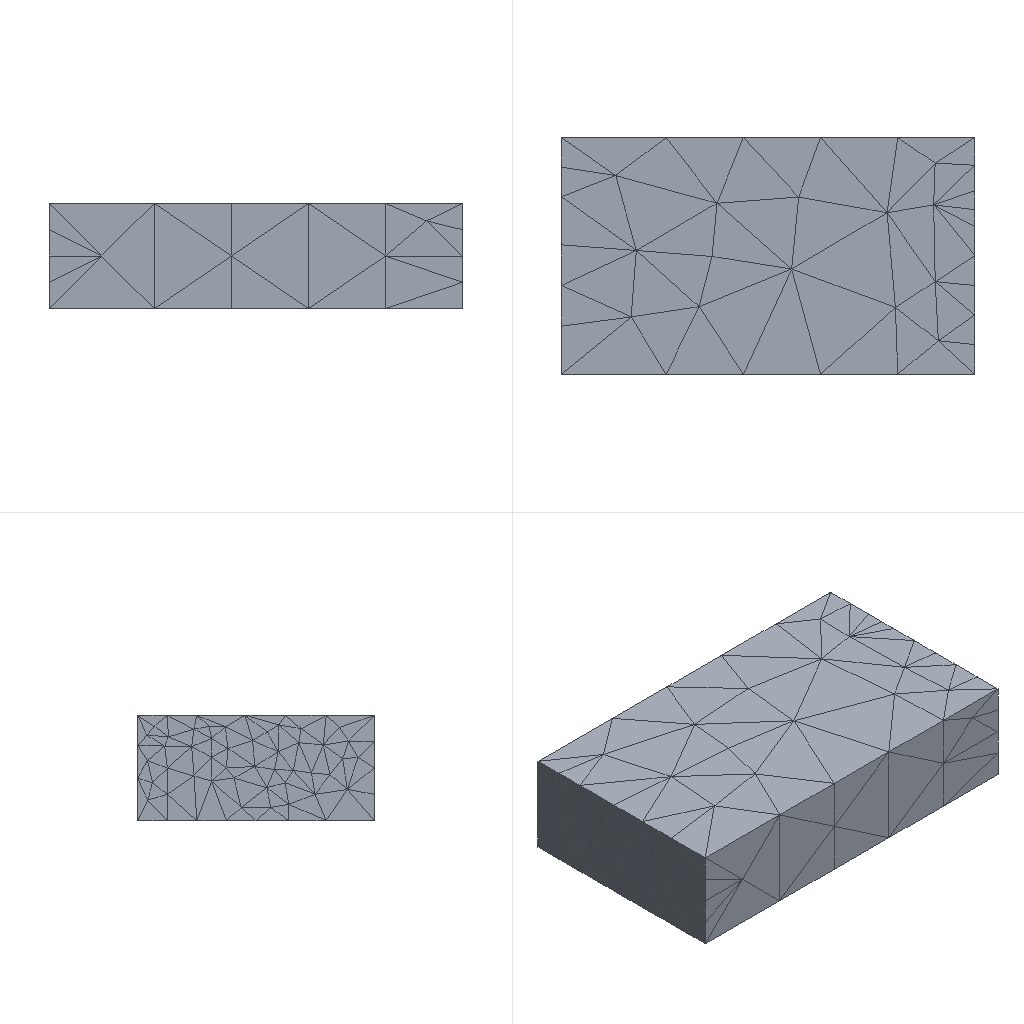Simulation study | ansys electronics desktop
Set-up summary:
category,name,step,type,value,unit,region
solver,ansys_electronics_desktop
units,length mm,,stated,model units
analysis,M03,,HFSS Modal Network,design_type=HFSS
setup,Setup1,M03,HfssDriven,frequency=10GHz; max_passes=2; max_delta_s=0.08
sweep,Sweep1,Setup1,Interpolating,8GHz..12GHz n=11 step=
mesh,nodes,,,n/a (no mesh stored)
mesh,elements,,,n/a (no mesh stored)
material,vacuum,,permittivity,1
load,P1,M03,wave port,,,objects 34
load,P2,M03,wave port,,,objects 46
bc,PerfE_6CU0FH,M03,perfect e,,,objects 58
bc,PerfE_674NPD,M03,perfect e,,,objects 70
bc,PerfE_5CT5JI,M03,perfect e,,,objects 82
bc,PerfE_WCUXQC,M03,perfect e,,,objects 94
Ansys Electronics Desktop project file, long lists of numbers shortened, first 681 of 3480 lines:
$begin 'AnsoftProject'
	Created='Wed Sep 30 18:28:02 2026'
	Product='ElectronicsDesktop'
	FileOwnedByWorkbench=false
	$begin 'Desktop'
		Version(2026, 1)
		InfrastructureVersion(1, 0)
		$begin 'FactoryHeader'
			$begin 'geometry3deditor'
				KernelVersion(2, 0)
				ProjectContainsGeometry3D='1'
			$end 'geometry3deditor'
		$end 'FactoryHeader'
	$end 'Desktop'
	UsesAdvancedFeatures=false
	PreviewImageDesignId=1
	NextUniqueID=0
	MoveBackwards=false
	$begin 'HFSSEnvironment'
		Version(1, 0)
	$end 'HFSSEnvironment'
	$begin 'PlanarEMEnvironment'
		Version(1, 0)
	$end 'PlanarEMEnvironment'
	$begin 'Q3DEnvironment'
		Version(1, 0)
	$end 'Q3DEnvironment'
	$begin '2DExtractorEnvironment'
		Version(1, 0)
	$end '2DExtractorEnvironment'
	$begin 'NexximEnvironment'
		Version(1, 0)
	$end 'NexximEnvironment'
	$begin 'NexximNetlistEnvironment'
		Version(1, 0)
	$end 'NexximNetlistEnvironment'
	$begin 'EmitEnvironment'
		Version(1, 0)
	$end 'EmitEnvironment'
	$begin 'Maxwell3DEnvironment'
		Version(1, 0)
	$end 'Maxwell3DEnvironment'
	$begin 'Maxwell2DEnvironment'
		Version(1, 0)
	$end 'Maxwell2DEnvironment'
	$begin 'RMxprtEnvironment'
		Version(1, 0)
	$end 'RMxprtEnvironment'
	$begin 'MaxCirEnvironment'
		Version(1, 0)
	$end 'MaxCirEnvironment'
	$begin 'SimplorerEnvironment'
		Version(1, 0)
	$end 'SimplorerEnvironment'
	$begin 'IcepakEnvironment'
		Version(1, 0)
	$end 'IcepakEnvironment'
	$begin 'IcepakFEAEnvironment'
		Version(1, 0)
	$end 'IcepakFEAEnvironment'
	$begin 'SchematicEnvironment'
		Version(1, 0)
	$end 'SchematicEnvironment'
	$begin 'geometry3deditor'
		Version(1, 0)
	$end 'geometry3deditor'
	ReadVersion=12
	$begin 'DesignMgrEnvironment'
		CompInstCounter=1
		GPortCounter=0
		NetCounter=0
		Alias('Ieee;Simplorer Elements\\Ieee', 'Std;Simplorer Elements\\Std', 'Basic_VHDLAMS;Simplorer Elements\\Basic Elements VHDLAMS\\Basic Elements VHDLAMS', 'Digital_Elements;Simplorer Elements\\Digital Elements\\Digital Elements', 'Transformations;Simplorer Elements\\Tools\\Transformations\\Transformations', 'HEV_VHDLAMS;Simplorer Elements\\HEV VHDLAMS\\HEV VHDLAMS', 'automotive_vda;Simplorer Elem
	$end 'DesignMgrEnvironment'
	$begin 'ProjectDatasets'
		NextUniqueID=0
		MoveBackwards=false
		DatasetType='ProjectDatasetType'
		$begin 'DatasetDefinitions'
		$end 'DatasetDefinitions'
	$end 'ProjectDatasets'
	VariableOrders[0:]
	$begin 'Definitions'
		$begin 'Materials'
			$begin 'vacuum'
				CoordinateSystemType='Cartesian'
				BulkOrSurfaceType=1
				$begin 'PhysicsTypes'
					set('Electromagnetic')
				$end 'PhysicsTypes'
				$begin 'AttachedData'
					$begin 'MatAppearanceData'
						property_data='appearance_data'
						Red=230
						Green=230
						Blue=230
						Transparency=0.95
					$end 'MatAppearanceData'
				$end 'AttachedData'
				permittivity='1'
				ModTime=1499970477
				Library='Materials'
				LibLocation='SysLibrary'
				ModSinceLib=false
			$end 'vacuum'
		$end 'Materials'
		$begin 'SurfaceMaterials'
		$end 'SurfaceMaterials'
		$begin 'Scripts'
		$end 'Scripts'
		$begin 'AnsysComponents'
			NextUniqueID=0
			MoveBackwards=false
			$begin 'AnsysComponentDefinitions'
			$end 'AnsysComponentDefinitions'
		$end 'AnsysComponents'
		$begin 'Symbols'
			$begin 'M03'
				ModTime=1790764083
				Library=''
				ModSinceLib=false
				LibLocation='Project'
				HighestLevel=1
				Normalize=true
				InitialLevels(0, 1)
				$begin 'Graphics'
					Rect(0, 0, 0, 0, 0.00254, 0.00254, 0.00508, 0.00508, 0, 0, 0)
					Rect(0, 1, 0, 0, 0.0004233, 0.00254, 0.0004233, 0.0004233, 0, 0, 0)
				$end 'Graphics'
			$end 'M03'
		$end 'Symbols'
		$begin 'DefInfo'
			M03(1002, 0, 0, 0, '', 1790764083, '', 'M03', '', '', '', '', '', 'Design.bmp', '', 'Project', '', '', 1790764083, '', 0, 0)
		$end 'DefInfo'
		$begin 'Compdefs'
			$begin 'M03'
				Library=''
				CircuitEnv=0
				Refbase='U'
				NumParts=1
				ModSinceLib=true
				$begin 'Properties'
					TextProp('Representation', 'SRD', '', 'M03')
					TextProp('Owner', 'SRD', '', 'HFSS')
				$end 'Properties'
				CompExtID=6
				$begin 'Parameters'
					ButtonProp('CosimDefinition', 'D', '', 'Edit', 'Edit', 40501, ButtonPropClientData())
					MenuProp('CoSimulator', 'D', '', 'DefaultNetlist', 0)
				$end 'Parameters'
				$begin 'CosimDefinitions'
					$begin 'CosimDefinition'
						CosimulatorType=4
						CosimDefName='DefaultNetlist'
						IsDefinition=true
						Connect=true
						Data()
						GRef()
					$end 'CosimDefinition'
					DefaultCosim='DefaultNetlist'
				$end 'CosimDefinitions'
			$end 'M03'
		$end 'Compdefs'
	$end 'Definitions'
	DesignIDServer=2
	MoveBackwards=false
	$begin 'HFSSModel'
		RepRewriteV2=true
		Name='M03'
		DesignID=0
		'Use Advanced DC Extrapolation'=false
		'Use Power S'=false
		'Export FRTM After Simulation'=false
		'Export Rays After Simulation'=false
		'Export After Simulation'=false
		'Allow Material Override'=false
		'Calculate Lossy Dielectrics'=false
		'Perform Minimal validation'=false
		$begin 'TemperatureSettings'
			IncludeTemperatureDependence=false
			EnableFeedback=false
			Temperatures(6, '22cel', 34, '22cel', 46, '22cel', 58, '22cel', 70, '22cel', 82, '22cel', 94, '22cel')
		$end 'TemperatureSettings'
		ObjsEnabledForDeformation()
		'Port Validation Settings'='Standard'
		'Save Adaptive support files'=false
		SolutionType='HFSS Modal Network'
		$begin 'DrivenOptions'
			AutoOpen=false
		$end 'DrivenOptions'
		HasTransientSetups=false
		MaterialDensity=1
		MassOfTissue=1
		VoxelSize=1
		TissueObjectList=-1
		AverageSarMethod=0
		UseAutoDCThickness=true
		HaveZwaveSupport=true
		SolveInsideThreshold=100000
		RequireBodyFaceInfo=false
		$begin 'OutputVariable'
			NextUniqueID=0
			MoveBackwards=false
		$end 'OutputVariable'
		$begin 'ModelSetup'
			$begin 'DesignDatasets'
				NextUniqueID=0
				MoveBackwards=false
				DatasetType='DesignDatasetType'
				$begin 'DatasetDefinitions'
				$end 'DatasetDefinitions'
			$end 'DesignDatasets'
			VariableOrders[0:]
			$begin 'Editor3D Doc Preferences'
				BackgroundColorVersion=1
				'Plane Background'=0
				'Need Lights'=true
				'Ambient Light'=8355711
				'Num Lights'=1
				Light0[4: 16777215, 0.75, -0.15, -0.63]
				Ver=2
			$end 'Editor3D Doc Preferences'
			SnapMode=31
			WorkingCS=1
			$begin 'GeometryCore'
				BlockVersionID=3
				DataVersion=2
				NativeKernel='PARASOLID'
				NativeKernelVersionID=26
				Units='mm'
				ModelExtents=10000
				InstanceID=-1
				$begin 'ValidationOptions'
					EntityCheckLevel='Strict'
					IgnoreUnclassifiedObjects=false
					SkipIntersectionChecks=false
				$end 'ValidationOptions'
				ContainsGeomLinkUDM=false
				$begin 'GeometryOperations'
					BlockVersionID=2
					$begin 'AnsoftRangedIDServerManager'
						$begin 'AnsoftRangedIDServer'
							IDServerObjectTypeID=0
							IDServerRangeMin=0
							IDServerRangeMax=2146483647
							NextUniqueID=105
							MoveBackwards=false
						$end 'AnsoftRangedIDServer'
						$begin 'AnsoftRangedIDServer'
							IDServerObjectTypeID=1
							IDServerRangeMin=2146483648
							IDServerRangeMax=2146485547
							NextUniqueID=2146483654
							MoveBackwards=false
						$end 'AnsoftRangedIDServer'
					$end 'AnsoftRangedIDServerManager'
					StartBackGroundFaceID=2146483648
					$begin 'CoordinateSystems'
					$end 'CoordinateSystems'
					$begin 'OperandCSs'
					$end 'OperandCSs'
					$begin 'SubModelDefinitions'
					$end 'SubModelDefinitions'
					$begin 'Groups'
					$end 'Groups'
					$begin 'UserDefinedModels'
					$end 'UserDefinedModels'
					$begin 'OperandUserDefinedModels'
					$end 'OperandUserDefinedModels'
					$begin 'ToplevelParts'
						$begin 'GeometryPart'
							$begin 'Attributes'
								Name='WG'
								Flags=''
								Color='(230 230 230)'
								Transparency=0.8
								PartCoordinateSystem=1
								UDMId=-1
								GroupId=-1
								MaterialValue='"vacuum"'
								SurfaceMaterialValue='""'
								SolveInside=true
								ShellElement=false
								ShellElementThickness='0mm'
								ReferenceTemperature='20cel'
								IsMaterialEditable=true
								IsSurfaceMaterialEditable=true
								UseMaterialAppearance=false
								IsLightweight=false
								IsAlwaysHidden=false
							$end 'Attributes'
							$begin 'PhysicsAttributes'
								SuppressedForPhysics='False'
								SuppressedForPhysicsEditable=true
							$end 'PhysicsAttributes'
							$begin 'Operations'
								$begin 'Operation'
									OperationType='Box'
									ID=5
									ReferenceCoordSystemID=1
									$begin 'BoxParameters'
										KernelVersion=23
										XPosition='0mm'
										YPosition='0mm'
										ZPosition='0mm'
										XSize='40mm'
										YSize='22.86mm'
										ZSize='10.16mm'
									$end 'BoxParameters'
									ParentPartID=6
									ReferenceUDMID=-1
									IsSuppressed=false
									$begin 'OperationIdentity'
										$begin 'Topology'
											NumLumps=1
											NumShells=1
											NumFaces=6
											NumWires=0
											NumLoops=6
											NumCoedges=24
											NumEdges=12
											NumVertices=8
										$end 'Topology'
										BodyID=6
										StartFaceID=7
										StartEdgeID=13
										StartVertexID=25
										NumNewFaces=6
										NumNewEdges=12
										NumNewVertices=8
										FaceNameAndIDMap()
										EdgeNameAndIDMap()
										VertexNameAndIDMap()
									$end 'OperationIdentity'
								$end 'Operation'
							$end 'Operations'
							$begin 'SubregionDependencyInformation'
								ChildSubregions[0:]
							$end 'SubregionDependencyInformation'
						$end 'GeometryPart'
						$begin 'GeometryPart'
							$begin 'Attributes'
								Name='Port1'
								Flags=''
								Color='(230 230 230)'
								Transparency=0.8
								PartCoordinateSystem=1
								UDMId=-1
								GroupId=-1
								MaterialValue='"vacuum"'
								SurfaceMaterialValue='""'
								SolveInside=true
								ShellElement=false
								ShellElementThickness='0mm'
								ReferenceTemperature='20cel'
								IsMaterialEditable=true
								IsSurfaceMaterialEditable=true
								UseMaterialAppearance=false
								IsLightweight=false
								IsAlwaysHidden=false
							$end 'Attributes'
							$begin 'PhysicsAttributes'
								SuppressedForPhysics='False'
								SuppressedForPhysicsEditable=true
							$end 'PhysicsAttributes'
							$begin 'Operations'
								$begin 'Operation'
									OperationType='Rectangle'
									ID=33
									ReferenceCoordSystemID=1
									$begin 'RectangleParameters'
										KernelVersion=23
										XStart='0mm'
										YStart='0mm'
										ZStart='0mm'
										Width='22.86mm'
										Height='10.16mm'
										WhichAxis='X'
									$end 'RectangleParameters'
									ParentPartID=34
									ReferenceUDMID=-1
									IsSuppressed=false
									$begin 'OperationIdentity'
										$begin 'Topology'
											NumLumps=1
											NumShells=1
											NumFaces=0
											NumWires=1
											NumLoops=0
											NumCoedges=0
											NumEdges=4
											NumVertices=4
										$end 'Topology'
										BodyID=34
										StartFaceID=-1
										StartEdgeID=35
										StartVertexID=39
										NumNewFaces=0
										NumNewEdges=4
										NumNewVertices=4
										FaceNameAndIDMap()
										EdgeNameAndIDMap()
										VertexNameAndIDMap()
									$end 'OperationIdentity'
								$end 'Operation'
								$begin 'Operation'
									OperationType='CoverLines'
									ID=43
									$begin 'LocalOperationParameters'
										KernelVersion=23
										LocalOpPart=34
									$end 'LocalOperationParameters'
									ParentPartID=34
									ReferenceUDMID=-1
									IsSuppressed=false
									$begin 'OperationIdentity'
										$begin 'Topology'
											NumLumps=1
											NumShells=1
											NumFaces=1
											NumWires=0
											NumLoops=1
											NumCoedges=4
											NumEdges=4
											NumVertices=4
										$end 'Topology'
										BodyID=-1
										StartFaceID=44
										StartEdgeID=-1
										StartVertexID=-1
										NumNewFaces=1
										NumNewEdges=0
										NumNewVertices=0
										FaceNameAndIDMap()
										EdgeNameAndIDMap()
										VertexNameAndIDMap()
										$begin 'GeomTopolBasedOperationIdentityHelper'
											$begin 'NewFaces'
												$begin 'Face'
													NormalizedSerialNum=0
													ID=44
													$begin 'FaceGeomTopol'
														FaceTopol(1, 4, 4, 4)
														$begin 'FaceGeometry'
															Area=232.258
															FcUVMid(1.51681195174844e-15, 11.43, 5.08)
															$begin 'FcTolVts'
																TolVt(0, 0, 0, 5e-07)
																TolVt(1.39977129142543e-15, 22.86, 5.07593966858622e-15, 5e-07)
																TolVt(3.03362390349689e-15, 22.86, 10.16, 5e-07)
																TolVt(1.63385261207146e-15, -2.25597318603832e-15, 10.16, 5e-07)
															$end 'FcTolVts'
														$end 'FaceGeometry'
													$end 'FaceGeomTopol'
												$end 'Face'
											$end 'NewFaces'
											$begin 'NewEdges'
											$end 'NewEdges'
											$begin 'NewVertices'
											$end 'NewVertices'
										$end 'GeomTopolBasedOperationIdentityHelper'
									$end 'OperationIdentity'
									ParentOperationID=33
								$end 'Operation'
							$end 'Operations'
							$begin 'SubregionDependencyInformation'
								ChildSubregions[0:]
							$end 'SubregionDependencyInformation'
						$end 'GeometryPart'
						$begin 'GeometryPart'
							$begin 'Attributes'
								Name='Port2'
								Flags=''
								Color='(230 230 230)'
								Transparency=0.8
								PartCoordinateSystem=1
								UDMId=-1
								GroupId=-1
								MaterialValue='"vacuum"'
								SurfaceMaterialValue='""'
								SolveInside=true
								ShellElement=false
								ShellElementThickness='0mm'
								ReferenceTemperature='20cel'
								IsMaterialEditable=true
								IsSurfaceMaterialEditable=true
								UseMaterialAppearance=false
								IsLightweight=false
								IsAlwaysHidden=false
							$end 'Attributes'
							$begin 'PhysicsAttributes'
								SuppressedForPhysics='False'
								SuppressedForPhysicsEditable=true
							$end 'PhysicsAttributes'
							$begin 'Operations'
								$begin 'Operation'
									OperationType='Rectangle'
									ID=45
									ReferenceCoordSystemID=1
									$begin 'RectangleParameters'
										KernelVersion=23
										XStart='40mm'
										YStart='0mm'
										ZStart='0mm'
										Width='22.86mm'
										Height='10.16mm'
										WhichAxis='X'
									$end 'RectangleParameters'
									ParentPartID=46
									ReferenceUDMID=-1
									IsSuppressed=false
									$begin 'OperationIdentity'
										$begin 'Topology'
											NumLumps=1
											NumShells=1
											NumFaces=0
											NumWires=1
											NumLoops=0
											NumCoedges=0
											NumEdges=4
											NumVertices=4
										$end 'Topology'
										BodyID=46
										StartFaceID=-1
										StartEdgeID=47
										StartVertexID=51
										NumNewFaces=0
										NumNewEdges=4
										NumNewVertices=4
										FaceNameAndIDMap()
										EdgeNameAndIDMap()
										VertexNameAndIDMap()
									$end 'OperationIdentity'
								$end 'Operation'
								$begin 'Operation'
									OperationType='CoverLines'
									ID=55
									$begin 'LocalOperationParameters'
										KernelVersion=23
										LocalOpPart=46
									$end 'LocalOperationParameters'
									ParentPartID=46
									ReferenceUDMID=-1
									IsSuppressed=false
									$begin 'OperationIdentity'
										$begin 'Topology'
											NumLumps=1
											NumShells=1
											NumFaces=1
											NumWires=0
											NumLoops=1
											NumCoedges=4
											NumEdges=4
											NumVertices=4
										$end 'Topology'
										BodyID=-1
										StartFaceID=56
										StartEdgeID=-1
										StartVertexID=-1
										NumNewFaces=1
										NumNewEdges=0
										NumNewVertices=0
										FaceNameAndIDMap()
										EdgeNameAndIDMap()
										VertexNameAndIDMap()
										$begin 'GeomTopolBasedOperationIdentityHelper'
											$begin 'NewFaces'
												$begin 'Face'
													NormalizedSerialNum=0
													ID=56
													$begin 'FaceGeomTopol'
														FaceTopol(1, 4, 4, 4)
														$begin 'FaceGeometry'
															Area=232.258
															FcUVMid(40, 11.43, 5.08)
															$begin 'FcTolVts'
																TolVt(40, 0, 0, 5e-07)
																TolVt(40, 22.86, 5.07593966858622e-15, 5e-07)
																TolVt(40, 22.86, 10.16, 5e-07)
																TolVt(40, -2.25597318603832e-15, 10.16, 5e-07)
															$end 'FcTolVts'
														$end 'FaceGeometry'
													$end 'FaceGeomTopol'
												$end 'Face'
											$end 'NewFaces'
											$begin 'NewEdges'
											$end 'NewEdges'
											$begin 'NewVertices'
											$end 'NewVertices'
										$end 'GeomTopolBasedOperationIdentityHelper'
									$end 'OperationIdentity'
									ParentOperationID=45
								$end 'Operation'
							$end 'Operations'
							$begin 'SubregionDependencyInformation'
								ChildSubregions[0:]
							$end 'SubregionDependencyInformation'
						$end 'GeometryPart'
						$begin 'GeometryPart'
							$begin 'Attributes'
								Name='Wall0'
								Flags=''
								Color='(230 230 230)'
								Transparency=0.8
								PartCoordinateSystem=1
								UDMId=-1
								GroupId=-1
								MaterialValue='"vacuum"'
								SurfaceMaterialValue='""'
								SolveInside=true
								ShellElement=false
								ShellElementThickness='0mm'
								ReferenceTemperature='20cel'
								IsMaterialEditable=true
								IsSurfaceMaterialEditable=true
								UseMaterialAppearance=false
								IsLightweight=false
								IsAlwaysHidden=false
							$end 'Attributes'
							$begin 'PhysicsAttributes'
								SuppressedForPhysics='False'
								SuppressedForPhysicsEditable=true
							$end 'PhysicsAttributes'
							$begin 'Operations'
								$begin 'Operation'
									OperationType='Rectangle'
									ID=57
									ReferenceCoordSystemID=1
									$begin 'RectangleParameters'
										KernelVersion=23
										XStart='0mm'
										YStart='0mm'
										ZStart='0mm'
										Width='40mm'
										Height='22.86mm'
										WhichAxis='Z'
									$end 'RectangleParameters'
									ParentPartID=58
									ReferenceUDMID=-1
									IsSuppressed=false
									$begin 'OperationIdentity'
										$begin 'Topology'
											NumLumps=1
											NumShells=1
											NumFaces=0
											NumWires=1
											NumLoops=0
											NumCoedges=0
											NumEdges=4
											NumVertices=4
										$end 'Topology'
										BodyID=58
										StartFaceID=-1
										StartEdgeID=59
										StartVertexID=63
										NumNewFaces=0
										NumNewEdges=4
										NumNewVertices=4
										FaceNameAndIDMap()
										EdgeNameAndIDMap()
										VertexNameAndIDMap()
									$end 'OperationIdentity'
								$end 'Operation'
								$begin 'Operation'
									OperationType='CoverLines'
									ID=67
									$begin 'LocalOperationParameters'
										KernelVersion=23
										LocalOpPart=58
									$end 'LocalOperationParameters'
									ParentPartID=58
									ReferenceUDMID=-1
									IsSuppressed=false
									$begin 'OperationIdentity'
										$begin 'Topology'
											NumLumps=1
											NumShells=1
											NumFaces=1
											NumWires=0
											NumLoops=1
											NumCoedges=4
											NumEdges=4
Last 1295 lines:
														NumberFormat='Auto'
														$begin 'TextFont'
															$begin 'FontAttribute'
																$begin 'Font'
																	HeightInPts=9
																	Width=0
																	Escapement=0
																	Orientation=0
																	Weight=400
																	Italic=0
																	Underline=0
																	StrikeOut=0
																	CharSet=0
																	OutPrecision=7
																	ClipPrecision=48
																	Quality=6
																	PitchAndFamily=0
																	FaceName='Arial'
																$end 'Font'
																ColorVersion=1
															$end 'FontAttribute'
														$end 'TextFont'
														InfMapMode=false
														InfMapValue=1.79769313486232e+306
														AutoRangeMin=true
														AutoRangeMax=true
														AutoSpacing=true
														kNumMinorDivisions=5
														ShowAxisTitle=true
														ShowAxisUnits=true
														vwm='FullWnd'
														viewWndWd=#nan
														ActivateMargins=true
														MarginPercent=0
														NeverCollapse=false
														AxisStripes=true
													$end 'LineAxisRenderAttribute'
												$end 'SubMapItem'
												$begin 'SubMapItem'
													DataSourceID=2
													$begin 'LineAxisRenderAttribute'
														DecimalFieldWidth=3
														DecimalFieldPrecision=2
														ManualTitle=''
														ColorVersion=1
														MinScale=0
														MaxScale=1
														TickSpacing=1
														ManualUnits=false
														Units='mm'
														AxisScale='Linear'
														NumberFormat='Auto'
														$begin 'TextFont'
															$begin 'FontAttribute'
																$begin 'Font'
																	HeightInPts=9
																	Width=0
																	Escapement=0
																	Orientation=0
																	Weight=400
																	Italic=0
																	Underline=0
																	StrikeOut=0
																	CharSet=0
																	OutPrecision=7
																	ClipPrecision=48
																	Quality=6
																	PitchAndFamily=0
																	FaceName='Arial'
																$end 'Font'
																ColorVersion=1
															$end 'FontAttribute'
														$end 'TextFont'
														InfMapMode=false
														InfMapValue=1.79769313486232e+306
														AutoRangeMin=true
														AutoRangeMax=true
														AutoSpacing=true
														kNumMinorDivisions=5
														ShowAxisTitle=true
														ShowAxisUnits=true
														vwm='FullWnd'
														viewWndWd=#nan
														ActivateMargins=true
														MarginPercent=0
														NeverCollapse=false
														AxisStripes=true
													$end 'LineAxisRenderAttribute'
												$end 'SubMapItem'
												$begin 'SubMapItem'
													DataSourceID=8
													$begin 'LineAxisRenderAttribute'
														DecimalFieldWidth=3
														DecimalFieldPrecision=2
														ManualTitle=''
														ColorVersion=1
														MinScale=0
														MaxScale=1
														TickSpacing=1
														ManualUnits=false
														Units='mm'
														AxisScale='Linear'
														NumberFormat='Auto'
														$begin 'TextFont'
															$begin 'FontAttribute'
																$begin 'Font'
																	HeightInPts=9
																	Width=0
																	Escapement=0
																	Orientation=0
																	Weight=400
																	Italic=0
																	Underline=0
																	StrikeOut=0
																	CharSet=0
																	OutPrecision=7
																	ClipPrecision=48
																	Quality=6
																	PitchAndFamily=0
																	FaceName='Arial'
																$end 'Font'
																ColorVersion=1
															$end 'FontAttribute'
														$end 'TextFont'
														InfMapMode=false
														InfMapValue=1.79769313486232e+306
														AutoRangeMin=true
														AutoRangeMax=true
														AutoSpacing=true
														kNumMinorDivisions=5
														ShowAxisTitle=true
														ShowAxisUnits=true
														vwm='FullWnd'
														viewWndWd=#nan
														ActivateMargins=true
														MarginPercent=0
														NeverCollapse=false
														AxisStripes=true
													$end 'LineAxisRenderAttribute'
												$end 'SubMapItem'
												$begin 'SubMapItem'
													DataSourceID=9
													$begin 'LineAxisRenderAttribute'
														DecimalFieldWidth=3
														DecimalFieldPrecision=2
														ManualTitle=''
														ColorVersion=1
														MinScale=0
														MaxScale=1
														TickSpacing=1
														ManualUnits=false
														Units='mm'
														AxisScale='Linear'
														NumberFormat='Auto'
														$begin 'TextFont'
															$begin 'FontAttribute'
																$begin 'Font'
																	HeightInPts=9
																	Width=0
																	Escapement=0
																	Orientation=0
																	Weight=400
																	Italic=0
																	Underline=0
																	StrikeOut=0
																	CharSet=0
																	OutPrecision=7
																	ClipPrecision=48
																	Quality=6
																	PitchAndFamily=0
																	FaceName='Arial'
																$end 'Font'
																ColorVersion=1
															$end 'FontAttribute'
														$end 'TextFont'
														InfMapMode=false
														InfMapValue=1.79769313486232e+306
														AutoRangeMin=true
														AutoRangeMax=true
														AutoSpacing=true
														kNumMinorDivisions=5
														ShowAxisTitle=true
														ShowAxisUnits=true
														vwm='FullWnd'
														viewWndWd=#nan
														ActivateMargins=true
														MarginPercent=0
														NeverCollapse=false
														AxisStripes=true
													$end 'LineAxisRenderAttribute'
												$end 'SubMapItem'
												$begin 'SubMapItem'
													DataSourceID=10
													$begin 'LineAxisRenderAttribute'
														DecimalFieldWidth=3
														DecimalFieldPrecision=2
														ManualTitle=''
														ColorVersion=1
														MinScale=0
														MaxScale=1
														TickSpacing=1
														ManualUnits=false
														Units='mm'
														AxisScale='Linear'
														NumberFormat='Auto'
														$begin 'TextFont'
															$begin 'FontAttribute'
																$begin 'Font'
																	HeightInPts=9
																	Width=0
																	Escapement=0
																	Orientation=0
																	Weight=400
																	Italic=0
																	Underline=0
																	StrikeOut=0
																	CharSet=0
																	OutPrecision=7
																	ClipPrecision=48
																	Quality=6
																	PitchAndFamily=0
																	FaceName='Arial'
																$end 'Font'
																ColorVersion=1
															$end 'FontAttribute'
														$end 'TextFont'
														InfMapMode=false
														InfMapValue=1.79769313486232e+306
														AutoRangeMin=true
														AutoRangeMax=true
														AutoSpacing=true
														kNumMinorDivisions=5
														ShowAxisTitle=true
														ShowAxisUnits=true
														vwm='FullWnd'
														viewWndWd=#nan
														ActivateMargins=true
														MarginPercent=0
														NeverCollapse=false
														AxisStripes=true
													$end 'LineAxisRenderAttribute'
												$end 'SubMapItem'
												$begin 'SubMapItem'
													DataSourceID=11
													$begin 'LineAxisRenderAttribute'
														DecimalFieldWidth=3
														DecimalFieldPrecision=2
														ManualTitle=''
														ColorVersion=1
														MinScale=0
														MaxScale=1
														TickSpacing=1
														ManualUnits=false
														Units='mm'
														AxisScale='Linear'
														NumberFormat='Auto'
														$begin 'TextFont'
															$begin 'FontAttribute'
																$begin 'Font'
																	HeightInPts=9
																	Width=0
																	Escapement=0
																	Orientation=0
																	Weight=400
																	Italic=0
																	Underline=0
																	StrikeOut=0
																	CharSet=0
																	OutPrecision=7
																	ClipPrecision=48
																	Quality=6
																	PitchAndFamily=0
																	FaceName='Arial'
																$end 'Font'
																ColorVersion=1
															$end 'FontAttribute'
														$end 'TextFont'
														InfMapMode=false
														InfMapValue=1.79769313486232e+306
														AutoRangeMin=true
														AutoRangeMax=true
														AutoSpacing=true
														kNumMinorDivisions=5
														ShowAxisTitle=true
														ShowAxisUnits=true
														vwm='FullWnd'
														viewWndWd=#nan
														ActivateMargins=true
														MarginPercent=0
														NeverCollapse=false
														AxisStripes=true
													$end 'LineAxisRenderAttribute'
												$end 'SubMapItem'
												$begin 'SubMapItem'
													DataSourceID=12
													$begin 'LineAxisRenderAttribute'
														DecimalFieldWidth=3
														DecimalFieldPrecision=2
														ManualTitle=''
														ColorVersion=1
														MinScale=0
														MaxScale=1
														TickSpacing=1
														ManualUnits=false
														Units='mm'
														AxisScale='Linear'
														NumberFormat='Auto'
														$begin 'TextFont'
															$begin 'FontAttribute'
																$begin 'Font'
																	HeightInPts=9
																	Width=0
																	Escapement=0
																	Orientation=0
																	Weight=400
																	Italic=0
																	Underline=0
																	StrikeOut=0
																	CharSet=0
																	OutPrecision=7
																	ClipPrecision=48
																	Quality=6
																	PitchAndFamily=0
																	FaceName='Arial'
																$end 'Font'
																ColorVersion=1
															$end 'FontAttribute'
														$end 'TextFont'
														InfMapMode=false
														InfMapValue=1.79769313486232e+306
														AutoRangeMin=true
														AutoRangeMax=true
														AutoSpacing=true
														kNumMinorDivisions=5
														ShowAxisTitle=true
														ShowAxisUnits=true
														vwm='FullWnd'
														viewWndWd=#nan
														ActivateMargins=true
														MarginPercent=0
														NeverCollapse=false
														AxisStripes=true
													$end 'LineAxisRenderAttribute'
												$end 'SubMapItem'
												$begin 'SubMapItem'
													DataSourceID=13
													$begin 'LineAxisRenderAttribute'
														DecimalFieldWidth=3
														DecimalFieldPrecision=2
														ManualTitle=''
														ColorVersion=1
														MinScale=0
														MaxScale=1
														TickSpacing=1
														ManualUnits=false
														Units='mm'
														AxisScale='Linear'
														NumberFormat='Auto'
														$begin 'TextFont'
															$begin 'FontAttribute'
																$begin 'Font'
																	HeightInPts=9
																	Width=0
																	Escapement=0
																	Orientation=0
																	Weight=400
																	Italic=0
																	Underline=0
																	StrikeOut=0
																	CharSet=0
																	OutPrecision=7
																	ClipPrecision=48
																	Quality=6
																	PitchAndFamily=0
																	FaceName='Arial'
																$end 'Font'
																ColorVersion=1
															$end 'FontAttribute'
														$end 'TextFont'
														InfMapMode=false
														InfMapValue=1.79769313486232e+306
														AutoRangeMin=true
														AutoRangeMax=true
														AutoSpacing=true
														kNumMinorDivisions=5
														ShowAxisTitle=true
														ShowAxisUnits=true
														vwm='FullWnd'
														viewWndWd=#nan
														ActivateMargins=true
														MarginPercent=0
														NeverCollapse=false
														AxisStripes=true
													$end 'LineAxisRenderAttribute'
												$end 'SubMapItem'
												$begin 'SubMapItem'
													DataSourceID=14
													$begin 'LineAxisRenderAttribute'
														DecimalFieldWidth=3
														DecimalFieldPrecision=2
														ManualTitle=''
														ColorVersion=1
														MinScale=0
														MaxScale=1
														TickSpacing=1
														ManualUnits=false
														Units='mm'
														AxisScale='Linear'
														NumberFormat='Auto'
														$begin 'TextFont'
															$begin 'FontAttribute'
																$begin 'Font'
																	HeightInPts=9
																	Width=0
																	Escapement=0
																	Orientation=0
																	Weight=400
																	Italic=0
																	Underline=0
																	StrikeOut=0
																	CharSet=0
																	OutPrecision=7
																	ClipPrecision=48
																	Quality=6
																	PitchAndFamily=0
																	FaceName='Arial'
																$end 'Font'
																ColorVersion=1
															$end 'FontAttribute'
														$end 'TextFont'
														InfMapMode=false
														InfMapValue=1.79769313486232e+306
														AutoRangeMin=true
														AutoRangeMax=true
														AutoSpacing=true
														kNumMinorDivisions=5
														ShowAxisTitle=true
														ShowAxisUnits=true
														vwm='FullWnd'
														viewWndWd=#nan
														ActivateMargins=true
														MarginPercent=0
														NeverCollapse=false
														AxisStripes=true
													$end 'LineAxisRenderAttribute'
												$end 'SubMapItem'
												$begin 'SubMapItem'
													DataSourceID=15
													$begin 'LineAxisRenderAttribute'
														DecimalFieldWidth=3
														DecimalFieldPrecision=2
														ManualTitle=''
														ColorVersion=1
														MinScale=0
														MaxScale=1
														TickSpacing=1
														ManualUnits=false
														Units='mm'
														AxisScale='Linear'
														NumberFormat='Auto'
														$begin 'TextFont'
															$begin 'FontAttribute'
																$begin 'Font'
																	HeightInPts=9
																	Width=0
																	Escapement=0
																	Orientation=0
																	Weight=400
																	Italic=0
																	Underline=0
																	StrikeOut=0
																	CharSet=0
																	OutPrecision=7
																	ClipPrecision=48
																	Quality=6
																	PitchAndFamily=0
																	FaceName='Arial'
																$end 'Font'
																ColorVersion=1
															$end 'FontAttribute'
														$end 'TextFont'
														InfMapMode=false
														InfMapValue=1.79769313486232e+306
														AutoRangeMin=true
														AutoRangeMax=true
														AutoSpacing=true
														kNumMinorDivisions=5
														ShowAxisTitle=true
														ShowAxisUnits=true
														vwm='FullWnd'
														viewWndWd=#nan
														ActivateMargins=true
														MarginPercent=0
														NeverCollapse=false
														AxisStripes=true
													$end 'LineAxisRenderAttribute'
												$end 'SubMapItem'
												$begin 'SubMapItem'
													DataSourceID=16
													$begin 'LineAxisRenderAttribute'
														DecimalFieldWidth=3
														DecimalFieldPrecision=2
														ManualTitle=''
														ColorVersion=1
														MinScale=0
														MaxScale=1
														TickSpacing=1
														ManualUnits=false
														Units='mm'
														AxisScale='Linear'
														NumberFormat='Auto'
														$begin 'TextFont'
															$begin 'FontAttribute'
																$begin 'Font'
																	HeightInPts=9
																	Width=0
																	Escapement=0
																	Orientation=0
																	Weight=400
																	Italic=0
																	Underline=0
																	StrikeOut=0
																	CharSet=0
																	OutPrecision=7
																	ClipPrecision=48
																	Quality=6
																	PitchAndFamily=0
																	FaceName='Arial'
																$end 'Font'
																ColorVersion=1
															$end 'FontAttribute'
														$end 'TextFont'
														InfMapMode=false
														InfMapValue=1.79769313486232e+306
														AutoRangeMin=true
														AutoRangeMax=true
														AutoSpacing=true
														kNumMinorDivisions=5
														ShowAxisTitle=true
														ShowAxisUnits=true
														vwm='FullWnd'
														viewWndWd=#nan
														ActivateMargins=true
														MarginPercent=0
														NeverCollapse=false
														AxisStripes=true
													$end 'LineAxisRenderAttribute'
												$end 'SubMapItem'
												$begin 'SubMapItem'
													DataSourceID=17
													$begin 'LineAxisRenderAttribute'
														DecimalFieldWidth=3
														DecimalFieldPrecision=2
														ManualTitle=''
														ColorVersion=1
														MinScale=0
														MaxScale=1
														TickSpacing=1
														ManualUnits=false
														Units='mm'
														AxisScale='Linear'
														NumberFormat='Auto'
														$begin 'TextFont'
															$begin 'FontAttribute'
																$begin 'Font'
																	HeightInPts=9
																	Width=0
																	Escapement=0
																	Orientation=0
																	Weight=400
																	Italic=0
																	Underline=0
																	StrikeOut=0
																	CharSet=0
																	OutPrecision=7
																	ClipPrecision=48
																	Quality=6
																	PitchAndFamily=0
																	FaceName='Arial'
																$end 'Font'
																ColorVersion=1
															$end 'FontAttribute'
														$end 'TextFont'
														InfMapMode=false
														InfMapValue=1.79769313486232e+306
														AutoRangeMin=true
														AutoRangeMax=true
														AutoSpacing=true
														kNumMinorDivisions=5
														ShowAxisTitle=true
														ShowAxisUnits=true
														vwm='FullWnd'
														viewWndWd=#nan
														ActivateMargins=true
														MarginPercent=0
														NeverCollapse=false
														AxisStripes=true
													$end 'LineAxisRenderAttribute'
												$end 'SubMapItem'
												$begin 'SubMapItem'
													DataSourceID=18
													$begin 'LineAxisRenderAttribute'
														DecimalFieldWidth=3
														DecimalFieldPrecision=2
														ManualTitle=''
														ColorVersion=1
														MinScale=0
														MaxScale=1
														TickSpacing=1
														ManualUnits=false
														Units='mm'
														AxisScale='Linear'
														NumberFormat='Auto'
														$begin 'TextFont'
															$begin 'FontAttribute'
																$begin 'Font'
																	HeightInPts=9
																	Width=0
																	Escapement=0
																	Orientation=0
																	Weight=400
																	Italic=0
																	Underline=0
																	StrikeOut=0
																	CharSet=0
																	OutPrecision=7
																	ClipPrecision=48
																	Quality=6
																	PitchAndFamily=0
																	FaceName='Arial'
																$end 'Font'
																ColorVersion=1
															$end 'FontAttribute'
														$end 'TextFont'
														InfMapMode=false
														InfMapValue=1.79769313486232e+306
														AutoRangeMin=true
														AutoRangeMax=true
														AutoSpacing=true
														kNumMinorDivisions=5
														ShowAxisTitle=true
														ShowAxisUnits=true
														vwm='FullWnd'
														viewWndWd=#nan
														ActivateMargins=true
														MarginPercent=0
														NeverCollapse=false
														AxisStripes=true
													$end 'LineAxisRenderAttribute'
												$end 'SubMapItem'
												$begin 'SubMapItem'
													DataSourceID=19
													$begin 'LineAxisRenderAttribute'
														DecimalFieldWidth=3
														DecimalFieldPrecision=2
														ManualTitle=''
														ColorVersion=1
														MinScale=0
														MaxScale=1
														TickSpacing=1
														ManualUnits=false
														Units='mm'
														AxisScale='Linear'
														NumberFormat='Auto'
														$begin 'TextFont'
															$begin 'FontAttribute'
																$begin 'Font'
																	HeightInPts=9
																	Width=0
																	Escapement=0
																	Orientation=0
																	Weight=400
																	Italic=0
																	Underline=0
																	StrikeOut=0
																	CharSet=0
																	OutPrecision=7
																	ClipPrecision=48
																	Quality=6
																	PitchAndFamily=0
																	FaceName='Arial'
																$end 'Font'
																ColorVersion=1
															$end 'FontAttribute'
														$end 'TextFont'
														InfMapMode=false
														InfMapValue=1.79769313486232e+306
														AutoRangeMin=true
														AutoRangeMax=true
														AutoSpacing=true
														kNumMinorDivisions=5
														ShowAxisTitle=true
														ShowAxisUnits=true
														vwm='FullWnd'
														viewWndWd=#nan
														ActivateMargins=true
														MarginPercent=0
														NeverCollapse=false
														AxisStripes=true
													$end 'LineAxisRenderAttribute'
												$end 'SubMapItem'
												$begin 'SubMapItem'
													DataSourceID=20
													$begin 'LineAxisRenderAttribute'
														DecimalFieldWidth=3
														DecimalFieldPrecision=2
														ManualTitle=''
														ColorVersion=1
														MinScale=0
														MaxScale=1
														TickSpacing=1
														ManualUnits=false
														Units='mm'
														AxisScale='Linear'
														NumberFormat='Auto'
														$begin 'TextFont'
															$begin 'FontAttribute'
																$begin 'Font'
																	HeightInPts=9
																	Width=0
																	Escapement=0
																	Orientation=0
																	Weight=400
																	Italic=0
																	Underline=0
																	StrikeOut=0
																	CharSet=0
																	OutPrecision=7
																	ClipPrecision=48
																	Quality=6
																	PitchAndFamily=0
																	FaceName='Arial'
																$end 'Font'
																ColorVersion=1
															$end 'FontAttribute'
														$end 'TextFont'
														InfMapMode=false
														InfMapValue=1.79769313486232e+306
														AutoRangeMin=true
														AutoRangeMax=true
														AutoSpacing=true
														kNumMinorDivisions=5
														ShowAxisTitle=true
														ShowAxisUnits=true
														vwm='FullWnd'
														viewWndWd=#nan
														ActivateMargins=true
														MarginPercent=0
														NeverCollapse=false
														AxisStripes=true
													$end 'LineAxisRenderAttribute'
												$end 'SubMapItem'
												$begin 'SubMapItem'
													DataSourceID=21
													$begin 'LineAxisRenderAttribute'
														DecimalFieldWidth=3
														DecimalFieldPrecision=2
														ManualTitle=''
														ColorVersion=1
														MinScale=0
														MaxScale=1
														TickSpacing=1
														ManualUnits=false
														Units='mm'
														AxisScale='Linear'
														NumberFormat='Auto'
														$begin 'TextFont'
															$begin 'FontAttribute'
																$begin 'Font'
																	HeightInPts=9
																	Width=0
																	Escapement=0
																	Orientation=0
																	Weight=400
																	Italic=0
																	Underline=0
																	StrikeOut=0
																	CharSet=0
																	OutPrecision=7
																	ClipPrecision=48
																	Quality=6
																	PitchAndFamily=0
																	FaceName='Arial'
																$end 'Font'
																ColorVersion=1
															$end 'FontAttribute'
														$end 'TextFont'
														InfMapMode=false
														InfMapValue=1.79769313486232e+306
														AutoRangeMin=true
														AutoRangeMax=true
														AutoSpacing=true
														kNumMinorDivisions=5
														ShowAxisTitle=true
														ShowAxisUnits=true
														vwm='FullWnd'
														viewWndWd=#nan
														ActivateMargins=true
														MarginPercent=0
														NeverCollapse=false
														AxisStripes=true
													$end 'LineAxisRenderAttribute'
												$end 'SubMapItem'
												$begin 'SubMapItem'
													DataSourceID=22
													$begin 'LineAxisRenderAttribute'
														DecimalFieldWidth=3
														DecimalFieldPrecision=2
														ManualTitle=''
														ColorVersion=1
														MinScale=0
														MaxScale=1
														TickSpacing=1
														ManualUnits=false
														Units='mm'
														AxisScale='Linear'
														NumberFormat='Auto'
														$begin 'TextFont'
															$begin 'FontAttribute'
																$begin 'Font'
																	HeightInPts=9
																	Width=0
																	Escapement=0
																	Orientation=0
																	Weight=400
																	Italic=0
																	Underline=0
																	StrikeOut=0
																	CharSet=0
																	OutPrecision=7
																	ClipPrecision=48
																	Quality=6
																	PitchAndFamily=0
																	FaceName='Arial'
																$end 'Font'
																ColorVersion=1
															$end 'FontAttribute'
														$end 'TextFont'
														InfMapMode=false
														InfMapValue=1.79769313486232e+306
														AutoRangeMin=true
														AutoRangeMax=true
														AutoSpacing=true
														kNumMinorDivisions=5
														ShowAxisTitle=true
														ShowAxisUnits=true
														vwm='FullWnd'
														viewWndWd=#nan
														ActivateMargins=true
														MarginPercent=0
														NeverCollapse=false
														AxisStripes=true
													$end 'LineAxisRenderAttribute'
												$end 'SubMapItem'
												$begin 'SubMapItem'
													DataSourceID=23
													$begin 'LineAxisRenderAttribute'
														DecimalFieldWidth=3
														DecimalFieldPrecision=2
														ManualTitle=''
														ColorVersion=1
														MinScale=0
														MaxScale=1
														TickSpacing=1
														ManualUnits=false
														Units='mm'
														AxisScale='Linear'
														NumberFormat='Auto'
														$begin 'TextFont'
															$begin 'FontAttribute'
																$begin 'Font'
																	HeightInPts=9
																	Width=0
																	Escapement=0
																	Orientation=0
																	Weight=400
																	Italic=0
																	Underline=0
																	StrikeOut=0
																	CharSet=0
																	OutPrecision=7
																	ClipPrecision=48
																	Quality=6
																	PitchAndFamily=0
																	FaceName='Arial'
																$end 'Font'
																ColorVersion=1
															$end 'FontAttribute'
														$end 'TextFont'
														InfMapMode=false
														InfMapValue=1.79769313486232e+306
														AutoRangeMin=true
														AutoRangeMax=true
														AutoSpacing=true
														kNumMinorDivisions=5
														ShowAxisTitle=true
														ShowAxisUnits=true
														vwm='FullWnd'
														viewWndWd=#nan
														ActivateMargins=true
														MarginPercent=0
														NeverCollapse=false
														AxisStripes=true
													$end 'LineAxisRenderAttribute'
												$end 'SubMapItem'
												$begin 'SubMapItem'
													DataSourceID=24
													$begin 'LineAxisRenderAttribute'
														DecimalFieldWidth=3
														DecimalFieldPrecision=2
														ManualTitle=''
														ColorVersion=1
														MinScale=0
														MaxScale=1
														TickSpacing=1
														ManualUnits=false
														Units='mm'
														AxisScale='Linear'
														NumberFormat='Auto'
														$begin 'TextFont'
															$begin 'FontAttribute'
																$begin 'Font'
																	HeightInPts=9
																	Width=0
																	Escapement=0
																	Orientation=0
																	Weight=400
																	Italic=0
																	Underline=0
																	StrikeOut=0
																	CharSet=0
																	OutPrecision=7
																	ClipPrecision=48
																	Quality=6
																	PitchAndFamily=0
																	FaceName='Arial'
																$end 'Font'
																ColorVersion=1
															$end 'FontAttribute'
														$end 'TextFont'
														InfMapMode=false
														InfMapValue=1.79769313486232e+306
														AutoRangeMin=true
														AutoRangeMax=true
														AutoSpacing=true
														kNumMinorDivisions=5
														ShowAxisTitle=true
														ShowAxisUnits=true
														vwm='FullWnd'
														viewWndWd=#nan
														ActivateMargins=true
														MarginPercent=0
														NeverCollapse=false
														AxisStripes=true
													$end 'LineAxisRenderAttribute'
												$end 'SubMapItem'
												$begin 'SubMapItem'
													DataSourceID=25
													$begin 'LineAxisRenderAttribute'
														DecimalFieldWidth=3
														DecimalFieldPrecision=2
														ManualTitle=''
														ColorVersion=1
														MinScale=0
														MaxScale=1
														TickSpacing=1
														ManualUnits=false
														Units='mm'
														AxisScale='Linear'
														NumberFormat='Auto'
														$begin 'TextFont'
															$begin 'FontAttribute'
																$begin 'Font'
																	HeightInPts=9
																	Width=0
																	Escapement=0
																	Orientation=0
																	Weight=400
																	Italic=0
																	Underline=0
																	StrikeOut=0
																	CharSet=0
																	OutPrecision=7
																	ClipPrecision=48
																	Quality=6
																	PitchAndFamily=0
																	FaceName='Arial'
																$end 'Font'
																ColorVersion=1
															$end 'FontAttribute'
														$end 'TextFont'
														InfMapMode=false
														InfMapValue=1.79769313486232e+306
														AutoRangeMin=true
														AutoRangeMax=true
														AutoSpacing=true
														kNumMinorDivisions=5
														ShowAxisTitle=true
														ShowAxisUnits=true
														vwm='FullWnd'
														viewWndWd=#nan
														ActivateMargins=true
														MarginPercent=0
														NeverCollapse=false
														AxisStripes=true
													$end 'LineAxisRenderAttribute'
												$end 'SubMapItem'
												$begin 'SubMapItem'
													DataSourceID=26
													$begin 'LineAxisRenderAttribute'
														DecimalFieldWidth=3
														DecimalFieldPrecision=2
														ManualTitle=''
														ColorVersion=1
														MinScale=0
														MaxScale=1
														TickSpacing=1
														ManualUnits=false
														Units='mm'
														AxisScale='Linear'
														NumberFormat='Auto'
														$begin 'TextFont'
															$begin 'FontAttribute'
																$begin 'Font'
																	HeightInPts=9
																	Width=0
																	Escapement=0
																	Orientation=0
																	Weight=400
																	Italic=0
																	Underline=0
																	StrikeOut=0
																	CharSet=0
																	OutPrecision=7
																	ClipPrecision=48
																	Quality=6
																	PitchAndFamily=0
																	FaceName='Arial'
																$end 'Font'
																ColorVersion=1
															$end 'FontAttribute'
														$end 'TextFont'
														InfMapMode=false
														InfMapValue=1.79769313486232e+306
														AutoRangeMin=true
														AutoRangeMax=true
														AutoSpacing=true
														kNumMinorDivisions=5
														ShowAxisTitle=true
														ShowAxisUnits=true
														vwm='FullWnd'
														viewWndWd=#nan
														ActivateMargins=true
														MarginPercent=0
														NeverCollapse=false
														AxisStripes=true
													$end 'LineAxisRenderAttribute'
												$end 'SubMapItem'
											$end 'MainMapItem'
										$end 'PlotAttributeStoreMap'
									$end 'DisplayTypeAttributes'
									$begin 'DocDefaultAttributes'
										$begin 'PlotAttributeStoreMap'
										$end 'PlotAttributeStoreMap'
									$end 'DocDefaultAttributes'
									$begin 'PerViewPlotAttributeStoreMap'
										$begin 'MapItem'
											ItemID=-1
											$begin 'PlotAttributeStoreMap'
												$begin 'MainMapItem'
													$begin 'SubMapItem'
														DataSourceID=4
														$begin 'BasicLayoutAttribute'
															$begin 'LayoutRect'
																Top=898
																Left=1122
																Bottom=9763
																Right=8948
															$end 'LayoutRect'
														$end 'BasicLayoutAttribute'
													$end 'SubMapItem'
													$begin 'SubMapItem'
														DataSourceID=28
														$begin 'BasicLayoutAttribute'
															$begin 'LayoutRect'
																Top=898
																Left=1122
																Bottom=9763
																Right=8948
															$end 'LayoutRect'
														$end 'BasicLayoutAttribute'
													$end 'SubMapItem'
													$begin 'SubMapItem'
														DataSourceID=35
														$begin 'BasicLayoutAttribute'
															$begin 'LayoutRect'
																Top=75
																Left=75
																Bottom=9925
																Right=875
															$end 'LayoutRect'
														$end 'BasicLayoutAttribute'
													$end 'SubMapItem'
												$end 'MainMapItem'
												$begin 'MainMapItem'
													$begin 'SubMapItem'
														DataSourceID=31
														$begin 'CartesianAxisLayoutAttribute'
															$begin 'AxisRect'
																Top=75
																Left=8948
																Bottom=9925
																Right=9925
															$end 'AxisRect'
															$begin 'GridRect'
																Top=898
																Left=1122
																Bottom=9763
																Right=8948
															$end 'GridRect'
															AxisCollapsed=false
															AxisExpandCollapseByUser=false
														$end 'CartesianAxisLayoutAttribute'
													$end 'SubMapItem'
													$begin 'SubMapItem'
														DataSourceID=32
														$begin 'CartesianAxisLayoutAttribute'
															$begin 'AxisRect'
																Top=75
																Left=1122
																Bottom=898
																Right=8948
															$end 'AxisRect'
															$begin 'GridRect'
																Top=898
																Left=1122
																Bottom=9763
																Right=8948
															$end 'GridRect'
															AxisCollapsed=false
															AxisExpandCollapseByUser=false
														$end 'CartesianAxisLayoutAttribute'
													$end 'SubMapItem'
												$end 'MainMapItem'
												$begin 'MainMapItem'
													$begin 'SubMapItem'
														DataSourceID=4
														$begin 'CartesianCurveGroupLayoutAttribute'
															X_spc=500000000
															X_fwd=3
															X_fpr=1
															Y1_spc=2.5
															Y1_fwd=3
															Y1_fpr=1
														$end 'CartesianCurveGroupLayoutAttribute'
													$end 'SubMapItem'
												$end 'MainMapItem'
												$begin 'MainMapItem'
													$begin 'SubMapItem'
														DataSourceID=6
														$begin 'DockableOverlayLayoutAttribute'
															$begin 'Dock_0'
																$begin 'OverlayLayoutAttribute'
																	$begin 'BoundingRect'
																		Top=4850
																		Left=975
																		Bottom=9850
																		Right=8475
																	$end 'BoundingRect'
																	ModifySize=false
																	ModifyPosition=false
																$end 'OverlayLayoutAttribute'
															$end 'Dock_0'
															$begin 'Dock_1'
																$begin 'OverlayLayoutAttribute'
																	$begin 'BoundingRect'
																		Top=5000
																		Left=0
																		Bottom=10000
																		Right=10000
																	$end 'BoundingRect'
																	ModifySize=false
																	ModifyPosition=false
																$end 'OverlayLayoutAttribute'
															$end 'Dock_1'
															$begin 'Dock_2'
																$begin 'OverlayLayoutAttribute'
																	$begin 'BoundingRect'
																		Top=0
																		Left=0
																		Bottom=5000
																		Right=10000
																	$end 'BoundingRect'
																	ModifySize=false
																	ModifyPosition=false
																$end 'OverlayLayoutAttribute'
															$end 'Dock_2'
														$end 'DockableOverlayLayoutAttribute'
													$end 'SubMapItem'
												$end 'MainMapItem'
											$end 'PlotAttributeStoreMap'
											PlotType=1
										$end 'MapItem'
									$end 'PerViewPlotAttributeStoreMap'
									IsViewAttribServer=false
									ViewID=-1
									$begin 'SourceIDMap'
										IDMapItem(0, 0, -1, 37)
										IDMapItem(1, 0, -1, 39)
									$end 'SourceIDMap'
									$begin 'TraceCharacteristicsMgr'
									$end 'TraceCharacteristicsMgr'
									$begin 'CartesianXMarkerManager'
										RefMarkerID=-1
										CurrentMarkerID=-1
										$begin 'ReferenceCurves'
										$end 'ReferenceCurves'
									$end 'CartesianXMarkerManager'
									$begin 'CartesianYMarkerManager'
									$end 'CartesianYMarkerManager'
									XAxisStackID=-1
									$begin 'AllTransSrcDwg'
										$begin 'PT'
											ID=1
											TransSrcDwg(-1, 0, 35, 1, 31, 2, 32, 5, 6, 27, 28, 37, 38, 39, 40)
										$end 'PT'
									$end 'AllTransSrcDwg'
									$begin 'AllPtSVID'
										PtID(1, -1, 4)
									$end 'AllPtSVID'
								$end 'PlotDisplayDataManager'
							$end 'Report2D'
						$end 'S_Parameters'
					$end 'Reports'
					$begin 'ReportsWindowInfoList'
						$begin 'S_Parameters'
							ReportID=2
							$begin 'WindowInfoList'
							$end 'WindowInfoList'
						$end 'S_Parameters'
					$end 'ReportsWindowInfoList'
				$end 'ReportSetup'
				$begin 'Properties'
				$end 'Properties'
				$begin 'UserDefinedDocument'
					$begin 'Data'
					$end 'Data'
				$end 'UserDefinedDocument'
			$end 'HfssDesignInstance'
		$end 'Instance'
		$begin 'SODInfo'
			$begin 'M03'
				$begin 'CosimDefinition'
					CosimDefName='DefaultNetlist'
					$begin 'SODInstanceMap'
					$end 'SODInstanceMap'
					SODComponentList()
				$end 'CosimDefinition'
			$end 'M03'
		$end 'SODInfo'
	$end 'DataInstances'
	$begin 'WBSystemIDToDesignInstanceIDMap'
	$end 'WBSystemIDToDesignInstanceIDMap'
	$begin 'WBSysIDSysDetails'
	$end 'WBSysIDSysDetails'
	$begin 'WBConnIDConnDetails'
	$end 'WBConnIDConnDetails'
	$begin 'WBMaterialGuidDetails'
		WBMaterialGuidMap()
	$end 'WBMaterialGuidDetails'
	$begin 'MinervaProjectSettingsBlk'
		MinervaRemoteFilePath=''
		FolderContainerString=''
	$end 'MinervaProjectSettingsBlk'
$end 'AnsoftProject'
$begin 'AllReferencedFilesForProject'
$end 'AllReferencedFilesForProject'
$begin 'ProjectPreview'
	ProductName='ElectronicsDesktop'
	MajorVersion=2026
	MinorVersion=1
	IsEncrypted=false
	Thumbnail64=''
	$begin 'DesignInfo'
		DesignName='M03'
		Notes=''
		Factory='HFSS'
		IsSolved=true
		'Nominal Setups'[1: 'Setup1']
		'Nominal Setup Types'[1: '']
		'Optimetrics Setups'[0:]
		'Optimetrics Experiment Types'[0:]
		Image64=''
	$end 'DesignInfo'
$end 'ProjectPreview'
Results summary, first 70 of 144 lines:
result,designs[0].name,1.step,,M03
result,designs[0].design_type,1.step,,HFSS
result,designs[0].solution_type,1.step,,HFSS Modal Network
result,designs[0].setups[0].name,Setup1,,Setup1
result,designs[0].setups[0].SetupType,Setup1,,HfssDriven
result,designs[0].setups[0].SolveType,Setup1,,Single
result,designs[0].setups[0].Frequency,Setup1,,10GHz
result,designs[0].setups[0].MaximumPasses,Setup1,,2
result,designs[0].setups[0].MaxDeltaS,Setup1,,0.08
result,designs[0].setups[0].IsEnabled,Setup1,,true
result,designs[0].setups[0].sweeps[0].name,Sweep1,,Sweep1
result,designs[0].setups[0].sweeps[0].RangeType,Sweep1,,LinearCount
result,designs[0].setups[0].sweeps[0].RangeStart,Sweep1,,8GHz
result,designs[0].setups[0].sweeps[0].RangeEnd,Sweep1,,12GHz
result,designs[0].setups[0].sweeps[0].RangeCount,Sweep1,,11
result,designs[0].setups[0].sweeps[0].Type,Sweep1,,Interpolating
result,designs[0].setups[0].sweeps[0].IsEnabled,Sweep1,,true
result,designs[0].boundaries[0].name,PerfE_6CU0FH,,PerfE_6CU0FH
result,designs[0].boundaries[0].BoundType,PerfE_6CU0FH,,Perfect E
result,designs[0].boundaries[1].name,PerfE_674NPD,,PerfE_674NPD
result,designs[0].boundaries[1].BoundType,PerfE_674NPD,,Perfect E
result,designs[0].boundaries[2].name,PerfE_5CT5JI,,PerfE_5CT5JI
result,designs[0].boundaries[2].BoundType,PerfE_5CT5JI,,Perfect E
result,designs[0].boundaries[3].name,PerfE_WCUXQC,,PerfE_WCUXQC
result,designs[0].boundaries[3].BoundType,PerfE_WCUXQC,,Perfect E
result,designs[0].excitations[0].name,P1,,P1
result,designs[0].excitations[0].BoundType,P1,,Wave Port
result,designs[0].excitations[0].WavePortType,P1,,Modal
result,designs[0].excitations[0].NumModes,P1,,1
result,designs[0].excitations[1].name,P2,,P2
result,designs[0].excitations[1].BoundType,P2,,Wave Port
result,designs[0].excitations[1].WavePortType,P2,,Modal
result,designs[0].excitations[1].NumModes,P2,,1
result,designs[0].materials_assigned[0],1.step,,vacuum
result,designs[0].objects,1.step,,7
result,designs[0].model_units,1.step,,mm
result,designs[0].valid_solutions[0],1.step,,Setup1 : AdaptivePass
result,designs[0].valid_solutions[1],1.step,,Setup1 : LastAdaptive
result,designs[0].valid_solutions[2],1.step,,Setup1 : Sweep1
result,designs[0].sparams[0].freq_hz[1],1.step,,8e+09
result,designs[0].sparams[0].freq_hz[2],1.step,,8.4e+09
result,designs[0].sparams[0].freq_hz[3],1.step,,8.8e+09
result,designs[0].sparams[0].freq_hz[4],1.step,,9.2e+09
result,designs[0].sparams[0].freq_hz[5],1.step,,9.6e+09
result,designs[0].sparams[0].freq_hz[6],1.step,,1e+10
result,designs[0].sparams[0].freq_hz[7],1.step,,1.04e+10
result,designs[0].sparams[0].freq_hz[8],1.step,,1.08e+10
result,designs[0].sparams[0].freq_hz[9],1.step,,1.12e+10
result,designs[0].sparams[0].freq_hz[10],1.step,,1.16e+10
result,designs[0].sparams[0].freq_hz[11],1.step,,1.2e+10
result,designs[0].sparams[0].expr,1.step,,"dB(S(P1,P1))"
result,designs[0].sparams[0].min_db,1.step,,-19.567
result,designs[0].sparams[0].solution,1.step,,Setup1 : Sweep1
result,designs[0].sparams[0].value_db[1],1.step,,-0.7722
result,designs[0].sparams[0].value_db[2],1.step,,-0.4392
result,designs[0].sparams[0].value_db[3],1.step,,-0.4729
result,designs[0].sparams[0].value_db[4],1.step,,-0.8186
result,designs[0].sparams[0].value_db[5],1.step,,-2.65
result,designs[0].sparams[0].value_db[6],1.step,,-19.567
result,designs[0].sparams[0].value_db[7],1.step,,-2.365
result,designs[0].sparams[0].value_db[8],1.step,,-1.006
result,designs[0].sparams[0].value_db[9],1.step,,-0.7146
result,designs[0].sparams[0].value_db[10],1.step,,-0.7139
result,designs[0].sparams[0].value_db[11],1.step,,-0.9712
result,designs[0].sparams[0].max_db,1.step,,-0.4392
result,designs[0].sparams[1].freq_hz[1],1.step,,8e+09
result,designs[0].sparams[1].freq_hz[2],1.step,,8.4e+09
result,designs[0].sparams[1].freq_hz[3],1.step,,8.8e+09
result,designs[0].sparams[1].freq_hz[4],1.step,,9.2e+09
result,designs[0].sparams[1].freq_hz[5],1.step,,9.6e+09